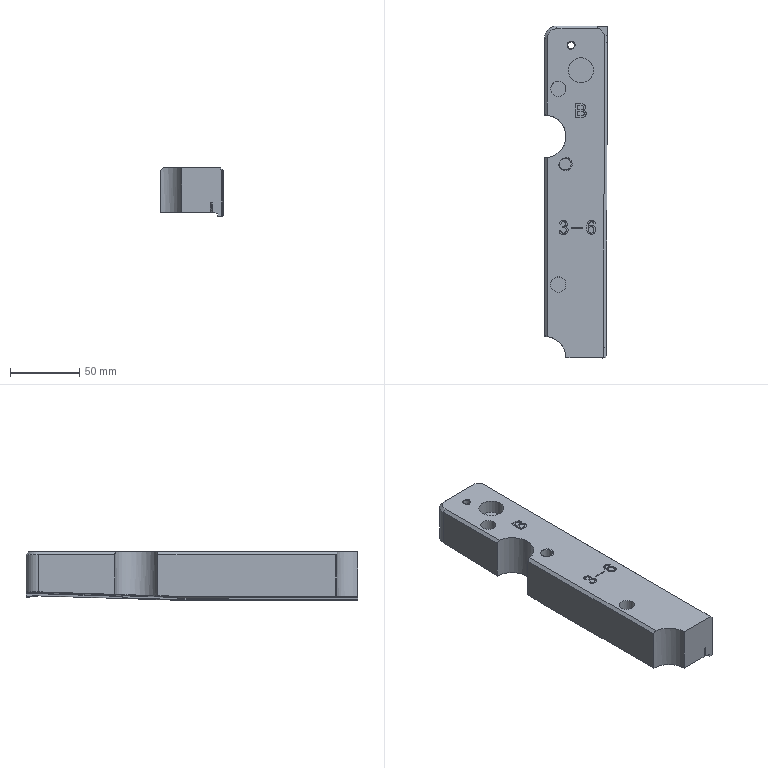NC program | NX | posted with a generic post | part box 45.476 x 239.737 x 35.001 mm
Lines 2815 to 3828 of 16758:
(HOLE_MILLING_1 , TOOL : D10)
N5628 M6
N5630 G53
N5632 G17 G0 G90 X-87.06 Y3.968 S3500 M3
N5634 G43 Z30. H0
N5636 G94 G1 Z0.23 F4000.
N5638 G3 X-87.869 Y7.473 Z0.2 R1.846 F1500.
N5640 X-87.869 Y7.473 Z0.05 I0. J-3.9
N5642 X-87.869 Y7.473 Z-0.1 I0. J-3.9
N5644 X-87.869 Y7.473 Z-0.25 I0. J-3.9
N5646 X-87.869 Y7.473 Z-0.4 I0. J-3.9
N5648 X-87.869 Y7.473 Z-0.55 I0. J-3.9
N5650 X-87.869 Y7.473 Z-0.7 I0. J-3.9
N5652 X-87.869 Y7.473 Z-0.85 I0. J-3.9
N5654 X-87.869 Y7.473 Z-1. I0. J-3.9
N5656 X-87.869 Y7.473 Z-1.15 I0. J-3.9
N5658 X-87.869 Y7.473 Z-1.3 I0. J-3.9
N5660 X-87.869 Y7.473 Z-1.45 I0. J-3.9
N5662 X-87.869 Y7.473 Z-1.6 I0. J-3.9
N5664 X-87.869 Y7.473 Z-1.75 I0. J-3.9
N5666 X-87.869 Y7.473 Z-1.9 I0. J-3.9
N5668 X-87.869 Y7.473 Z-2.05 I0. J-3.9
N5670 X-87.869 Y7.473 Z-2.2 I0. J-3.9
N5672 X-87.869 Y7.473 Z-2.35 I0. J-3.9
N5674 X-87.869 Y7.473 Z-2.5 I0. J-3.9
N5676 X-87.869 Y7.473 Z-2.65 I0. J-3.9
N5678 X-87.869 Y7.473 Z-2.8 I0. J-3.9
N5680 X-87.869 Y7.473 Z-2.95 I0. J-3.9
N5682 X-87.869 Y7.473 Z-3.1 I0. J-3.9
N5684 X-87.869 Y7.473 Z-3.25 I0. J-3.9
N5686 X-87.869 Y7.473 Z-3.4 I0. J-3.9
N5688 X-87.869 Y7.473 Z-3.55 I0. J-3.9
N5690 X-87.869 Y7.473 Z-3.7 I0. J-3.9
N5692 X-87.869 Y7.473 Z-3.85 I0. J-3.9
N5694 X-87.869 Y7.473 Z-4. I0. J-3.9
N5696 X-87.869 Y7.473 Z-4.15 I0. J-3.9
N5698 X-87.869 Y7.473 Z-4.3 I0. J-3.9
N5700 X-87.869 Y7.473 Z-4.45 I0. J-3.9
N5702 X-87.869 Y7.473 Z-4.6 I0. J-3.9
N5704 X-87.869 Y7.473 Z-4.75 I0. J-3.9
N5706 X-87.869 Y7.473 Z-4.9 I0. J-3.9
N5708 X-87.869 Y7.473 Z-5.05 I0. J-3.9
N5710 X-87.869 Y7.473 Z-5.2 I0. J-3.9
N5712 X-87.869 Y7.473 Z-5.35 I0. J-3.9
N5714 X-87.869 Y7.473 Z-5.5 I0. J-3.9
N5716 X-87.869 Y7.473 Z-5.65 I0. J-3.9
N5718 X-87.869 Y7.473 Z-5.8 I0. J-3.9
N5720 X-87.869 Y7.473 Z-5.95 I0. J-3.9
N5722 X-87.869 Y7.473 Z-6.1 I0. J-3.9
N5724 X-87.869 Y7.473 Z-6.25 I0. J-3.9
N5726 X-87.869 Y7.473 Z-6.4 I0. J-3.9
N5728 X-87.869 Y7.473 Z-6.55 I0. J-3.9
N5730 X-87.869 Y7.473 Z-6.7 I0. J-3.9
N5732 X-87.869 Y7.473 Z-6.85 I0. J-3.9
N5734 X-87.869 Y7.473 Z-7. I0. J-3.9
N5736 X-87.869 Y7.473 Z-7.15 I0. J-3.9
N5738 X-87.869 Y7.473 Z-7.3 I0. J-3.9
N5740 X-87.869 Y7.473 Z-7.45 I0. J-3.9
N5742 X-87.869 Y7.473 Z-7.6 I0. J-3.9
N5744 X-87.869 Y7.473 Z-7.75 I0. J-3.9
N5746 X-87.869 Y7.473 Z-7.9 I0. J-3.9
N5748 X-87.869 Y7.473 Z-8.05 I0. J-3.9
N5750 X-87.869 Y7.473 Z-8.2 I0. J-3.9
N5752 X-87.869 Y7.473 Z-8.35 I0. J-3.9
N5754 X-87.869 Y7.473 Z-8.5 I0. J-3.9
N5756 X-87.869 Y7.473 Z-8.65 I0. J-3.9
N5758 X-87.869 Y7.473 Z-8.8 I0. J-3.9
N5760 X-87.869 Y7.473 Z-8.95 I0. J-3.9
N5762 X-87.869 Y7.473 Z-9.1 I0. J-3.9
N5764 X-87.869 Y7.473 Z-9.25 I0. J-3.9
N5766 X-87.869 Y7.473 Z-9.4 I0. J-3.9
N5768 X-87.869 Y7.473 Z-9.55 I0. J-3.9
N5770 X-87.869 Y7.473 Z-9.7 I0. J-3.9
N5772 X-87.869 Y7.473 Z-9.85 I0. J-3.9
N5774 X-87.869 Y7.473 Z-10. I0. J-3.9
N5776 X-87.869 Y7.473 Z-10.15 I0. J-3.9
N5778 X-87.869 Y7.473 Z-10.3 I0. J-3.9
N5780 X-87.869 Y7.473 Z-10.45 I0. J-3.9
N5782 X-87.869 Y7.473 Z-10.6 I0. J-3.9
N5784 X-87.869 Y7.473 Z-10.75 I0. J-3.9
N5786 X-87.869 Y7.473 Z-10.9 I0. J-3.9
N5788 X-84.491 Y1.623 Z-11. R-3.9
N5790 X-85.919 Y6.951 R3.9
N5792 X-84.491 Y1.623 R-3.9
N5794 X-87.123 Y4.077 Z-10.936 R1.846
N5796 G0 Z30.
(HOLE_MILLING_1_COPY , TOOL : D10)
N5798 X-86.986 Y4.044
N5800 G1 Z0.23 F4000.
N5802 G3 X-87.869 Y7.573 Z0.2 R1.875 F1500.
N5804 X-87.869 Y7.573 Z0.05 I0. J-4.
N5806 X-87.869 Y7.573 Z-0.1 I0. J-4.
N5808 X-87.869 Y7.573 Z-0.25 I0. J-4.
N5810 X-87.869 Y7.573 Z-0.4 I0. J-4.
N5812 X-87.869 Y7.573 Z-0.55 I0. J-4.
N5814 X-87.869 Y7.573 Z-0.7 I0. J-4.
N5816 X-87.869 Y7.573 Z-0.85 I0. J-4.
N5818 X-87.869 Y7.573 Z-1. I0. J-4.
N5820 X-87.869 Y7.573 Z-1.15 I0. J-4.
N5822 X-87.869 Y7.573 Z-1.3 I0. J-4.
N5824 X-87.869 Y7.573 Z-1.45 I0. J-4.
N5826 X-87.869 Y7.573 Z-1.6 I0. J-4.
N5828 X-87.869 Y7.573 Z-1.75 I0. J-4.
N5830 X-87.869 Y7.573 Z-1.9 I0. J-4.
N5832 X-87.869 Y7.573 Z-2.05 I0. J-4.
N5834 X-87.869 Y7.573 Z-2.2 I0. J-4.
N5836 X-87.869 Y7.573 Z-2.35 I0. J-4.
N5838 X-87.869 Y7.573 Z-2.5 I0. J-4.
N5840 X-87.869 Y7.573 Z-2.65 I0. J-4.
N5842 X-87.869 Y7.573 Z-2.8 I0. J-4.
N5844 X-87.869 Y7.573 Z-2.95 I0. J-4.
N5846 X-87.869 Y7.573 Z-3.1 I0. J-4.
N5848 X-87.869 Y7.573 Z-3.25 I0. J-4.
N5850 X-87.869 Y7.573 Z-3.4 I0. J-4.
N5852 X-87.869 Y7.573 Z-3.55 I0. J-4.
N5854 X-87.869 Y7.573 Z-3.7 I0. J-4.
N5856 X-87.869 Y7.573 Z-3.85 I0. J-4.
N5858 X-87.869 Y7.573 Z-4. I0. J-4.
N5860 X-87.869 Y7.573 Z-4.15 I0. J-4.
N5862 X-87.869 Y7.573 Z-4.3 I0. J-4.
N5864 X-87.869 Y7.573 Z-4.45 I0. J-4.
N5866 X-87.869 Y7.573 Z-4.6 I0. J-4.
N5868 X-87.869 Y7.573 Z-4.75 I0. J-4.
N5870 X-87.869 Y7.573 Z-4.9 I0. J-4.
N5872 X-87.869 Y7.573 Z-5.05 I0. J-4.
N5874 X-87.869 Y7.573 Z-5.2 I0. J-4.
N5876 X-87.869 Y7.573 Z-5.35 I0. J-4.
N5878 X-87.869 Y7.573 Z-5.5 I0. J-4.
N5880 X-87.869 Y7.573 Z-5.65 I0. J-4.
N5882 X-87.869 Y7.573 Z-5.8 I0. J-4.
N5884 X-87.869 Y7.573 Z-5.95 I0. J-4.
N5886 X-87.869 Y7.573 Z-6.1 I0. J-4.
N5888 X-87.869 Y7.573 Z-6.25 I0. J-4.
N5890 X-87.869 Y7.573 Z-6.4 I0. J-4.
N5892 X-87.869 Y7.573 Z-6.55 I0. J-4.
N5894 X-87.869 Y7.573 Z-6.7 I0. J-4.
N5896 X-87.869 Y7.573 Z-6.85 I0. J-4.
N5898 X-87.869 Y7.573 Z-7. I0. J-4.
N5900 X-87.869 Y7.573 Z-7.15 I0. J-4.
N5902 X-87.869 Y7.573 Z-7.3 I0. J-4.
N5904 X-87.869 Y7.573 Z-7.45 I0. J-4.
N5906 X-87.869 Y7.573 Z-7.6 I0. J-4.
N5908 X-87.869 Y7.573 Z-7.75 I0. J-4.
N5910 X-87.869 Y7.573 Z-7.9 I0. J-4.
N5912 X-87.869 Y7.573 Z-8.05 I0. J-4.
N5914 X-87.869 Y7.573 Z-8.2 I0. J-4.
N5916 X-87.869 Y7.573 Z-8.35 I0. J-4.
N5918 X-87.869 Y7.573 Z-8.5 I0. J-4.
N5920 X-87.869 Y7.573 Z-8.65 I0. J-4.
N5922 X-87.869 Y7.573 Z-8.8 I0. J-4.
N5924 X-87.869 Y7.573 Z-8.95 I0. J-4.
N5926 X-87.869 Y7.573 Z-9.1 I0. J-4.
N5928 X-87.869 Y7.573 Z-9.25 I0. J-4.
N5930 X-87.869 Y7.573 Z-9.4 I0. J-4.
N5932 X-87.869 Y7.573 Z-9.55 I0. J-4.
N5934 X-87.869 Y7.573 Z-9.7 I0. J-4.
N5936 X-87.869 Y7.573 Z-9.85 I0. J-4.
N5938 X-87.869 Y7.573 Z-10. I0. J-4.
N5940 X-87.869 Y7.573 Z-10.15 I0. J-4.
N5942 X-91.333 Y1.573 Z-10.2 R4.
N5944 X-85.869 Y0.109 R4.
N5946 X-91.333 Y1.573 R-4.
N5948 X-87.835 Y2.574 Z-10.137 R1.875
N5950 G0 Z30.
(ZLEVEL_PROFILE_2 , TOOL : D10)
N5952 X-131.488 Y14.432 S3470
N5954 G1 Z0.1 F4000.
N5956 Z-0.1 F2000.
N5958 G3 X-127.246 Y14.432 R3.
N5960 G1 X-123.393 Y18.285
N5962 X-115.404 Y26.274
N5964 X-111.621 Y30.057
N5966 Z-0.2
N5968 X-115.404 Y26.274
N5970 X-123.393 Y18.285
N5972 X-127.246 Y14.432
N5974 Z-0.3
N5976 X-123.393 Y18.285
N5978 X-115.404 Y26.274
N5980 X-111.621 Y30.057
N5982 Z-0.4
N5984 X-115.404 Y26.274
N5986 X-123.393 Y18.285
N5988 X-127.246 Y14.432
N5990 Z-0.5
N5992 X-123.393 Y18.285
N5994 X-115.404 Y26.274
N5996 X-111.621 Y30.057
N5998 Z-0.6
N6000 X-115.404 Y26.274
N6002 X-123.393 Y18.285
N6004 X-127.246 Y14.432
N6006 Z-0.7
N6008 X-123.393 Y18.285
N6010 X-115.404 Y26.274
N6012 X-111.621 Y30.057
N6014 Z-0.8
N6016 X-115.404 Y26.274
N6018 X-123.393 Y18.285
N6020 X-127.246 Y14.432
N6022 Z-0.9
N6024 X-123.393 Y18.285
N6026 X-115.404 Y26.274
N6028 X-111.621 Y30.057
N6030 Z-1.
N6032 X-115.404 Y26.274
N6034 X-123.393 Y18.285
N6036 X-127.246 Y14.432
N6038 Z-1.1
N6040 X-123.393 Y18.285
N6042 X-115.404 Y26.274
N6044 X-111.621 Y30.057
N6046 Z-1.2
N6048 X-115.404 Y26.274
N6050 X-123.393 Y18.285
N6052 X-123.675 Y18.004
N6054 X-127.246 Y14.432
N6056 Z-1.3
N6058 X-123.675 Y18.004
N6060 X-123.393 Y18.285
N6062 X-115.404 Y26.274
N6064 X-111.622 Y30.057
N6066 Z-1.4
N6068 X-115.404 Y26.274
N6070 X-123.393 Y18.285
N6072 X-123.675 Y18.004
N6074 X-127.246 Y14.432
N6076 Z-1.5
N6078 X-123.675 Y18.004
N6080 X-123.393 Y18.285
N6082 X-115.404 Y26.274
N6084 X-111.622 Y30.057
N6086 Z-1.6
N6088 X-115.404 Y26.274
N6090 X-123.393 Y18.285
N6092 X-123.675 Y18.004
N6094 X-127.246 Y14.432
N6096 Z-1.7
N6098 X-123.675 Y18.004
N6100 X-123.393 Y18.285
N6102 X-115.404 Y26.274
N6104 X-111.622 Y30.057
N6106 Z-1.8
N6108 X-115.404 Y26.274
N6110 X-123.393 Y18.285
N6112 X-123.675 Y18.004
N6114 X-127.246 Y14.432
N6116 Z-1.9
N6118 X-123.675 Y18.004
N6120 X-123.393 Y18.285
N6122 X-115.404 Y26.274
N6124 X-111.622 Y30.057
N6126 Z-2.
N6128 X-115.404 Y26.274
N6130 X-123.404 Y18.274
N6132 X-123.451 Y18.227
N6134 X-127.246 Y14.432
N6136 Z-2.1
N6138 X-123.451 Y18.227
N6140 X-123.404 Y18.274
N6142 X-115.404 Y26.274
N6144 X-111.622 Y30.057
N6146 Z-2.2
N6148 X-115.404 Y26.274
N6150 X-123.404 Y18.274
N6152 X-123.451 Y18.227
N6154 X-126.859 Y14.819
N6156 X-127.246 Y14.432
N6158 Z-2.3
N6160 X-123.404 Y18.274
N6162 X-115.404 Y26.274
N6164 X-111.622 Y30.057
N6166 Z-2.4
N6168 X-115.404 Y26.274
N6170 X-123.404 Y18.274
N6172 X-127.246 Y14.432
N6174 Z-2.5
N6176 X-123.404 Y18.274
N6178 X-115.404 Y26.274
N6180 X-111.622 Y30.057
N6182 Z-2.6
N6184 X-115.404 Y26.274
N6186 X-123.404 Y18.274
N6188 X-127.246 Y14.432
N6190 Z-2.7
N6192 X-123.404 Y18.274
N6194 X-115.404 Y26.274
N6196 X-111.622 Y30.057
N6198 Z-2.8
N6200 X-115.404 Y26.274
N6202 X-123.404 Y18.274
N6204 X-127.246 Y14.432
N6206 Z-2.9
N6208 X-123.404 Y18.274
N6210 X-115.404 Y26.274
N6212 X-111.622 Y30.057
N6214 Z-3.
N6216 X-115.404 Y26.274
N6218 X-123.404 Y18.274
N6220 X-127.246 Y14.432
N6222 Z-3.1
N6224 X-123.404 Y18.274
N6226 X-115.404 Y26.274
N6228 X-111.622 Y30.057
N6230 Z-3.2
N6232 X-115.404 Y26.274
N6234 X-123.404 Y18.274
N6236 X-127.246 Y14.432
N6238 Z-3.3
N6240 X-123.404 Y18.274
N6242 X-115.404 Y26.274
N6244 X-111.622 Y30.057
N6246 Z-3.4
N6248 X-115.404 Y26.274
N6250 X-123.404 Y18.274
N6252 X-127.246 Y14.432
N6254 Z-3.5
N6256 X-123.404 Y18.274
N6258 X-115.404 Y26.274
N6260 X-111.622 Y30.057
N6262 Z-3.6
N6264 X-115.404 Y26.274
N6266 X-123.404 Y18.274
N6268 X-127.246 Y14.432
N6270 Z-3.7
N6272 X-123.404 Y18.274
N6274 X-115.404 Y26.274
N6276 X-111.622 Y30.057
N6278 Z-3.8
N6280 X-115.404 Y26.274
N6282 X-123.404 Y18.274
N6284 X-127.246 Y14.432
N6286 Z-3.9
N6288 X-123.404 Y18.274
N6290 X-115.404 Y26.274
N6292 X-111.622 Y30.057
N6294 Z-4.
N6296 X-115.404 Y26.274
N6298 X-123.404 Y18.274
N6300 X-127.246 Y14.432
N6302 Z-4.1
N6304 X-123.404 Y18.274
N6306 X-115.404 Y26.274
N6308 X-111.622 Y30.057
N6310 Z-4.2
N6312 X-115.404 Y26.274
N6314 X-123.404 Y18.274
N6316 X-127.246 Y14.432
N6318 Z-4.3
N6320 X-123.404 Y18.274
N6322 X-115.404 Y26.274
N6324 X-111.622 Y30.057
N6326 Z-4.4
N6328 X-115.404 Y26.274
N6330 X-123.404 Y18.274
N6332 X-127.246 Y14.432
N6334 Z-4.5
N6336 X-123.404 Y18.274
N6338 X-115.404 Y26.274
N6340 X-111.622 Y30.057
N6342 Z-4.6
N6344 X-115.404 Y26.274
N6346 X-123.404 Y18.274
N6348 X-127.246 Y14.432
N6350 Z-4.7
N6352 X-123.404 Y18.274
N6354 X-115.404 Y26.274
N6356 X-111.622 Y30.057
N6358 Z-4.8
N6360 X-115.404 Y26.274
N6362 X-123.404 Y18.274
N6364 X-127.246 Y14.432
N6366 Z-4.9
N6368 X-123.404 Y18.274
N6370 X-115.404 Y26.274
N6372 X-111.622 Y30.057
N6374 Z-5.
N6376 X-115.404 Y26.274
N6378 X-123.404 Y18.274
N6380 X-127.246 Y14.432
N6382 Z-5.1
N6384 X-123.404 Y18.274
N6386 X-115.404 Y26.274
N6388 X-111.622 Y30.057
N6390 Z-5.2
N6392 X-115.404 Y26.274
N6394 X-123.404 Y18.274
N6396 X-127.246 Y14.432
N6398 Z-5.3
N6400 X-123.404 Y18.274
N6402 X-115.404 Y26.274
N6404 X-111.622 Y30.057
N6406 Z-5.4
N6408 X-115.404 Y26.274
N6410 X-123.404 Y18.274
N6412 X-127.246 Y14.432
N6414 Z-5.5
N6416 X-123.404 Y18.274
N6418 X-115.404 Y26.274
N6420 X-111.622 Y30.057
N6422 G3 X-111.623 Y34.299 R3.
N6424 G1 Z-5.3
N6426 G0 Z30.
N6428 M5
(SPOT_DRILLING_1 , TOOL : Z3)
N6430 M6
N6432 G53
N6434 G17 G0 G90 X-105.869 Y-3.427 S3000 M3
N6436 G43 Z30. H0
N6438 G94 G81 G98 Z-1. F50. R1.
N6440 X-74.606 Y-12.738
N6442 X-20.131 Y-7.738
N6444 X66.869 Y-12.738
N6446 G80
N6448 G0 X66.869 Y-12.738 Z30.
N6450 M5
(SPOT_DRILLING_1_COPY , TOOL : Z8.5)
N6452 M6
N6454 G53
N6456 G17 G0 G90 X-74.606 Y-12.738 S600 M3
N6458 G43 Z30. H0
N6460 G94 G83 G98 Z-30. F50. Q2. R1.
N6462 X-20.131 Y-7.738
N6464 X66.869 Y-12.738
N6466 G80
N6468 G0 X66.869 Y-12.738 Z30.
N6470 M5
(PLANAR_TEXT_2 , TOOL : B1)
N6472 M6
N6474 G53
N6476 G17 G0 G90 X-13.566 Y8.073 S7500 M3
N6478 G43 Z30. H0
N6480 G94 G1 Z0.5 F4000.
N6482 Z-0.03 F750.
N6484 X-11.967 F1500.
N6486 X-10.92 Y7.286
N6488 Y5.002
N6490 X-11.967 Y4.294
N6492 X-14.117
N6494 X-15.109 Y5.002
N6496 Z0.47
N6498 G0 X-15.164 Y11.065 Z0.5
N6500 G1 Z-0.03 F750.
N6502 X-14.117 Y11.774 F1500.
N6504 X-11.967
N6506 X-10.92 Y11.065
N6508 Y8.782
N6510 X-11.967 Y8.073
N6512 Z0.47
N6514 G0 Z1.
N6516 X-6.562
N6518 G1 Z0.5 F4000.
N6520 Z-0.03 F750.
N6522 X-4.467 F1500.
N6524 Z0.47
N6526 G0 Z1.
N6528 X4.08 Y10.278
N6530 G1 Z0.5 F4000.
N6532 Z-0.03 F750.
N6534 X3.033 Y11.774 F1500.
N6536 X0.883
N6538 X-0.109 Y10.278
N6540 Y5.79
N6542 X0.883 Y4.294
N6544 X3.033
N6546 X4.08 Y5.79
N6548 Y7.286
N6550 X3.033 Y8.782
N6552 X0.883
N6554 X-0.109 Y7.286
N6556 Z0.47
N6558 G0 Z1.
N6560 X25.533 Y8.782
N6562 G1 Z0.5 F4000.
N6564 Z-0.03 F750.
N6566 X26.525 Y8.073 F1500.
N6568 Y5.002
N6570 X25.477 Y4.294
N6572 X22.391
N6574 Y8.782
N6576 X25.533
N6578 X26.029 Y9.569
N6580 Y11.065
N6582 X25.533 Y11.774
N6584 X22.391
N6586 Y8.782
N6588 Z0.47
N6590 G0 Z1.
N6592 X-13.566 Y8.073
N6594 G1 Z0.47 F4000.
N6596 Z-0.06 F750.
N6598 X-11.967 F1500.
N6600 X-10.92 Y7.286
N6602 Y5.002
N6604 X-11.967 Y4.294
N6606 X-14.117
N6608 X-15.109 Y5.002
N6610 Z0.44
N6612 G0 X-15.164 Y11.065 Z0.47
N6614 G1 Z-0.06 F750.
N6616 X-14.117 Y11.774 F1500.
N6618 X-11.967
N6620 X-10.92 Y11.065
N6622 Y8.782
N6624 X-11.967 Y8.073
N6626 Z0.44
N6628 G0 Z1.
N6630 X-6.562
N6632 G1 Z0.47 F4000.
N6634 Z-0.06 F750.
N6636 X-4.467 F1500.
N6638 Z0.44
N6640 G0 Z1.
N6642 X4.08 Y10.278
N6644 G1 Z0.47 F4000.
N6646 Z-0.06 F750.
N6648 X3.033 Y11.774 F1500.
N6650 X0.883
N6652 X-0.109 Y10.278
N6654 Y5.79
N6656 X0.883 Y4.294
N6658 X3.033
N6660 X4.08 Y5.79
N6662 Y7.286
N6664 X3.033 Y8.782
N6666 X0.883
N6668 X-0.109 Y7.286
N6670 Z0.44
N6672 G0 Z1.
N6674 X25.533 Y8.782
N6676 G1 Z0.47 F4000.
N6678 Z-0.06 F750.
N6680 X26.525 Y8.073 F1500.
N6682 Y5.002
N6684 X25.477 Y4.294
N6686 X22.391
N6688 Y8.782
N6690 X25.533
N6692 X26.029 Y9.569
N6694 Y11.065
N6696 X25.533 Y11.774
N6698 X22.391
N6700 Y8.782
N6702 Z0.44
N6704 G0 Z1.
N6706 X-13.566 Y8.073
N6708 G1 Z0.44 F4000.
N6710 Z-0.09 F750.
N6712 X-11.967 F1500.
N6714 X-10.92 Y7.286
N6716 Y5.002
N6718 X-11.967 Y4.294
N6720 X-14.117
N6722 X-15.109 Y5.002
N6724 Z0.41
N6726 G0 X-15.164 Y11.065 Z0.44
N6728 G1 Z-0.09 F750.
N6730 X-14.117 Y11.774 F1500.
N6732 X-11.967
N6734 X-10.92 Y11.065
N6736 Y8.782
N6738 X-11.967 Y8.073
N6740 Z0.41
N6742 G0 Z1.
N6744 X-6.562
N6746 G1 Z0.44 F4000.
N6748 Z-0.09 F750.
N6750 X-4.467 F1500.
N6752 Z0.41
N6754 G0 Z1.
N6756 X4.08 Y10.278
N6758 G1 Z0.44 F4000.
N6760 Z-0.09 F750.
N6762 X3.033 Y11.774 F1500.
N6764 X0.883
N6766 X-0.109 Y10.278
N6768 Y5.79
N6770 X0.883 Y4.294
N6772 X3.033
N6774 X4.08 Y5.79
N6776 Y7.286
N6778 X3.033 Y8.782
N6780 X0.883
N6782 X-0.109 Y7.286
N6784 Z0.41
N6786 G0 Z1.
N6788 X25.533 Y8.782
N6790 G1 Z0.44 F4000.
N6792 Z-0.09 F750.
N6794 X26.525 Y8.073 F1500.
N6796 Y5.002
N6798 X25.477 Y4.294
N6800 X22.391
N6802 Y8.782
N6804 X25.533
N6806 X26.029 Y9.569
N6808 Y11.065
N6810 X25.533 Y11.774
N6812 X22.391
N6814 Y8.782
N6816 Z0.41
N6818 G0 Z1.
N6820 X-13.566 Y8.073
N6822 G1 Z0.41 F4000.
N6824 Z-0.12 F750.
N6826 X-11.967 F1500.
N6828 X-10.92 Y7.286
N6830 Y5.002
N6832 X-11.967 Y4.294
N6834 X-14.117
N6836 X-15.109 Y5.002
N6838 Z0.38
N6840 G0 X-15.164 Y11.065 Z0.41
N6842 G1 Z-0.12 F750.
N6844 X-14.117 Y11.774 F1500.
N6846 X-11.967
N6848 X-10.92 Y11.065
N6850 Y8.782
N6852 X-11.967 Y8.073
N6854 Z0.38
N6856 G0 Z1.
N6858 X-6.562
N6860 G1 Z0.41 F4000.
N6862 Z-0.12 F750.
N6864 X-4.467 F1500.
N6866 Z0.38
N6868 G0 Z1.
N6870 X4.08 Y10.278
N6872 G1 Z0.41 F4000.
N6874 Z-0.12 F750.
N6876 X3.033 Y11.774 F1500.
N6878 X0.883
N6880 X-0.109 Y10.278
N6882 Y5.79
N6884 X0.883 Y4.294
N6886 X3.033
N6888 X4.08 Y5.79
N6890 Y7.286
N6892 X3.033 Y8.782
N6894 X0.883
N6896 X-0.109 Y7.286
N6898 Z0.38
N6900 G0 Z1.
N6902 X25.533 Y8.782
N6904 G1 Z0.41 F4000.
N6906 Z-0.12 F750.
N6908 X26.525 Y8.073 F1500.
N6910 Y5.002
N6912 X25.477 Y4.294
N6914 X22.391
N6916 Y8.782
N6918 X25.533
N6920 X26.029 Y9.569
N6922 Y11.065
N6924 X25.533 Y11.774
N6926 X22.391
N6928 Y8.782
N6930 Z0.38
N6932 G0 Z1.
N6934 X-13.566 Y8.073
N6936 G1 Z0.38 F4000.
N6938 Z-0.15 F750.
N6940 X-11.967 F1500.
N6942 X-10.92 Y7.286
N6944 Y5.002
N6946 X-11.967 Y4.294
N6948 X-14.117
N6950 X-15.109 Y5.002
N6952 Z0.35
N6954 G0 X-15.164 Y11.065 Z0.38
N6956 G1 Z-0.15 F750.
N6958 X-14.117 Y11.774 F1500.
N6960 X-11.967
N6962 X-10.92 Y11.065
N6964 Y8.782
N6966 X-11.967 Y8.073
N6968 Z0.35
N6970 G0 Z1.
N6972 X-6.562
N6974 G1 Z0.38 F4000.
N6976 Z-0.15 F750.
N6978 X-4.467 F1500.
N6980 Z0.35
N6982 G0 Z1.
N6984 X4.08 Y10.278
N6986 G1 Z0.38 F4000.
N6988 Z-0.15 F750.
N6990 X3.033 Y11.774 F1500.
N6992 X0.883
N6994 X-0.109 Y10.278
N6996 Y5.79
N6998 X0.883 Y4.294
N7000 X3.033
N7002 X4.08 Y5.79
N7004 Y7.286
N7006 X3.033 Y8.782
N7008 X0.883
N7010 X-0.109 Y7.286
N7012 Z0.35
N7014 G0 Z1.
N7016 X25.533 Y8.782
N7018 G1 Z0.38 F4000.
N7020 Z-0.15 F750.
N7022 X26.525 Y8.073 F1500.
N7024 Y5.002
N7026 X25.477 Y4.294
N7028 X22.391
N7030 Y8.782
N7032 X25.533
N7034 X26.029 Y9.569
N7036 Y11.065
N7038 X25.533 Y11.774
N7040 X22.391
N7042 Y8.782
N7044 Z0.35
N7046 G0 Z1.
N7048 X-13.566 Y8.073
N7050 G1 Z0.35 F4000.
N7052 Z-0.18 F750.
N7054 X-11.967 F1500.
N7056 X-10.92 Y7.286
N7058 Y5.002
N7060 X-11.967 Y4.294
N7062 X-14.117
N7064 X-15.109 Y5.002
N7066 Z0.32
N7068 G0 X-15.164 Y11.065 Z0.35
N7070 G1 Z-0.18 F750.
N7072 X-14.117 Y11.774 F1500.
N7074 X-11.967
N7076 X-10.92 Y11.065
N7078 Y8.782
N7080 X-11.967 Y8.073
N7082 Z0.32
N7084 G0 Z1.
N7086 X-6.562
N7088 G1 Z0.35 F4000.
N7090 Z-0.18 F750.
N7092 X-4.467 F1500.
N7094 Z0.32
N7096 G0 Z1.
N7098 X4.08 Y10.278
N7100 G1 Z0.35 F4000.
N7102 Z-0.18 F750.
N7104 X3.033 Y11.774 F1500.
N7106 X0.883
N7108 X-0.109 Y10.278
N7110 Y5.79
N7112 X0.883 Y4.294
N7114 X3.033
N7116 X4.08 Y5.79
N7118 Y7.286
N7120 X3.033 Y8.782
N7122 X0.883
N7124 X-0.109 Y7.286
N7126 Z0.32
N7128 G0 Z1.
N7130 X25.533 Y8.782
N7132 G1 Z0.35 F4000.
N7134 Z-0.18 F750.
N7136 X26.525 Y8.073 F1500.
N7138 Y5.002
N7140 X25.477 Y4.294
N7142 X22.391
N7144 Y8.782
N7146 X25.533
N7148 X26.029 Y9.569
N7150 Y11.065
N7152 X25.533 Y11.774
N7154 X22.391
N7156 Y8.782
N7158 Z0.32
N7160 G0 Z1.
N7162 X-13.566 Y8.073
N7164 G1 Z0.32 F4000.
N7166 Z-0.21 F750.
N7168 X-11.967 F1500.
N7170 X-10.92 Y7.286
N7172 Y5.002
N7174 X-11.967 Y4.294
N7176 X-14.117
N7178 X-15.109 Y5.002
N7180 Z0.29
N7182 G0 X-15.164 Y11.065 Z0.32
N7184 G1 Z-0.21 F750.
N7186 X-14.117 Y11.774 F1500.
N7188 X-11.967
N7190 X-10.92 Y11.065
N7192 Y8.782
N7194 X-11.967 Y8.073
N7196 Z0.29
N7198 G0 Z1.
N7200 X-6.562
N7202 G1 Z0.32 F4000.
N7204 Z-0.21 F750.
N7206 X-4.467 F1500.
N7208 Z0.29
N7210 G0 Z1.
N7212 X4.08 Y10.278
N7214 G1 Z0.32 F4000.
N7216 Z-0.21 F750.
N7218 X3.033 Y11.774 F1500.
N7220 X0.883
N7222 X-0.109 Y10.278
N7224 Y5.79
N7226 X0.883 Y4.294
N7228 X3.033
N7230 X4.08 Y5.79
N7232 Y7.286
N7234 X3.033 Y8.782
N7236 X0.883
N7238 X-0.109 Y7.286
N7240 Z0.29
N7242 G0 Z1.
N7244 X25.533 Y8.782
N7246 G1 Z0.32 F4000.
N7248 Z-0.21 F750.
N7250 X26.525 Y8.073 F1500.
N7252 Y5.002
N7254 X25.477 Y4.294
N7256 X22.391
N7258 Y8.782
N7260 X25.533
N7262 X26.029 Y9.569
N7264 Y11.065
N7266 X25.533 Y11.774
N7268 X22.391
N7270 Y8.782
N7272 Z0.29
N7274 G0 Z1.
N7276 X-13.566 Y8.073
N7278 G1 Z0.29 F4000.
N7280 Z-0.24 F750.
N7282 X-11.967 F1500.
N7284 X-10.92 Y7.286
N7286 Y5.002
N7288 X-11.967 Y4.294
N7290 X-14.117
N7292 X-15.109 Y5.002
N7294 Z0.26
N7296 G0 X-15.164 Y11.065 Z0.29
N7298 G1 Z-0.24 F750.
N7300 X-14.117 Y11.774 F1500.
N7302 X-11.967
N7304 X-10.92 Y11.065
N7306 Y8.782
N7308 X-11.967 Y8.073
N7310 Z0.26
N7312 G0 Z1.
N7314 X-6.562
N7316 G1 Z0.29 F4000.
N7318 Z-0.24 F750.
N7320 X-4.467 F1500.
N7322 Z0.26
N7324 G0 Z1.
N7326 X4.08 Y10.278
N7328 G1 Z0.29 F4000.
N7330 Z-0.24 F750.
N7332 X3.033 Y11.774 F1500.
N7334 X0.883
N7336 X-0.109 Y10.278
N7338 Y5.79
N7340 X0.883 Y4.294
N7342 X3.033
N7344 X4.08 Y5.79
N7346 Y7.286
N7348 X3.033 Y8.782
N7350 X0.883
N7352 X-0.109 Y7.286
N7354 Z0.26
N7356 G0 Z1.
N7358 X25.533 Y8.782
N7360 G1 Z0.29 F4000.
N7362 Z-0.24 F750.
N7364 X26.525 Y8.073 F1500.
N7366 Y5.002
N7368 X25.477 Y4.294
N7370 X22.391
N7372 Y8.782
N7374 X25.533
N7376 X26.029 Y9.569
N7378 Y11.065
N7380 X25.533 Y11.774
N7382 X22.391
N7384 Y8.782
N7386 Z0.26
N7388 G0 Z1.
N7390 X-13.566 Y8.073
N7392 G1 Z0.26 F4000.
N7394 Z-0.27 F750.
N7396 X-11.967 F1500.
N7398 X-10.92 Y7.286
N7400 Y5.002
N7402 X-11.967 Y4.294
N7404 X-14.117
N7406 X-15.109 Y5.002
N7408 Z0.23
N7410 G0 X-15.164 Y11.065 Z0.26
N7412 G1 Z-0.27 F750.
N7414 X-14.117 Y11.774 F1500.
N7416 X-11.967
N7418 X-10.92 Y11.065
N7420 Y8.782
N7422 X-11.967 Y8.073
N7424 Z0.23
N7426 G0 Z1.
N7428 X-6.562
N7430 G1 Z0.26 F4000.
N7432 Z-0.27 F750.
N7434 X-4.467 F1500.
N7436 Z0.23
N7438 G0 Z1.
N7440 X4.08 Y10.278
N7442 G1 Z0.26 F4000.
N7444 Z-0.27 F750.
N7446 X3.033 Y11.774 F1500.
N7448 X0.883
N7450 X-0.109 Y10.278
N7452 Y5.79
N7454 X0.883 Y4.294
N7456 X3.033
N7458 X4.08 Y5.79
N7460 Y7.286
N7462 X3.033 Y8.782
N7464 X0.883
N7466 X-0.109 Y7.286
N7468 Z0.23
N7470 G0 Z1.
N7472 X25.533 Y8.782
N7474 G1 Z0.26 F4000.
N7476 Z-0.27 F750.
N7478 X26.525 Y8.073 F1500.
N7480 Y5.002
N7482 X25.477 Y4.294
N7484 X22.391
N7486 Y8.782
N7488 X25.533
N7490 X26.029 Y9.569
N7492 Y11.065
N7494 X25.533 Y11.774
N7496 X22.391
N7498 Y8.782
N7500 Z0.23
N7502 G0 Z1.
N7504 X-13.566 Y8.073
N7506 G1 Z0.23 F4000.
N7508 Z-0.3 F750.
N7510 X-11.967 F1500.
N7512 X-10.92 Y7.286
N7514 Y5.002
N7516 X-11.967 Y4.294
N7518 X-14.117
N7520 X-15.109 Y5.002
N7522 Z0.2
N7524 G0 X-15.164 Y11.065 Z0.23
N7526 G1 Z-0.3 F750.
N7528 X-14.117 Y11.774 F1500.
N7530 X-11.967
N7532 X-10.92 Y11.065
N7534 Y8.782
N7536 X-11.967 Y8.073
N7538 Z0.2
N7540 G0 Z1.
N7542 X-6.562
N7544 G1 Z0.23 F4000.
N7546 Z-0.3 F750.
N7548 X-4.467 F1500.
N7550 Z0.2
N7552 G0 Z1.
N7554 X4.08 Y10.278
N7556 G1 Z0.23 F4000.
N7558 Z-0.3 F750.
N7560 X3.033 Y11.774 F1500.
N7562 X0.883
N7564 X-0.109 Y10.278
N7566 Y5.79
N7568 X0.883 Y4.294
N7570 X3.033
N7572 X4.08 Y5.79
N7574 Y7.286
N7576 X3.033 Y8.782
N7578 X0.883
N7580 X-0.109 Y7.286
N7582 Z0.2
N7584 G0 Z1.
N7586 X25.533 Y8.782
N7588 G1 Z0.23 F4000.
N7590 Z-0.3 F750.
N7592 X26.525 Y8.073 F1500.
N7594 Y5.002
N7596 X25.477 Y4.294
N7598 X22.391
N7600 Y8.782
N7602 X25.533
N7604 X26.029 Y9.569
N7606 Y11.065
N7608 X25.533 Y11.774
N7610 X22.391
N7612 Y8.782
N7614 Z0.2
N7616 G0 Z30.
N7618 M5